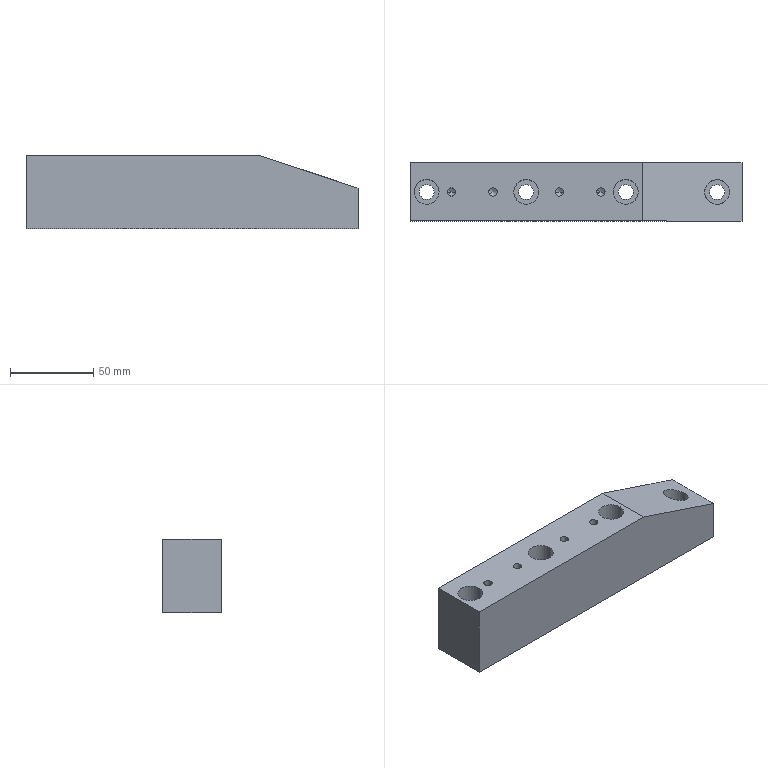Part | STEP file | connecting block | 1 solid | 43 faces | box 200 x 35 x 44.5 mm | volume 266252 mm3 | cylinder 24 | plane 11 | cone 8 | commonest cylinder face diameters 5 x8 9 x8 15 x8